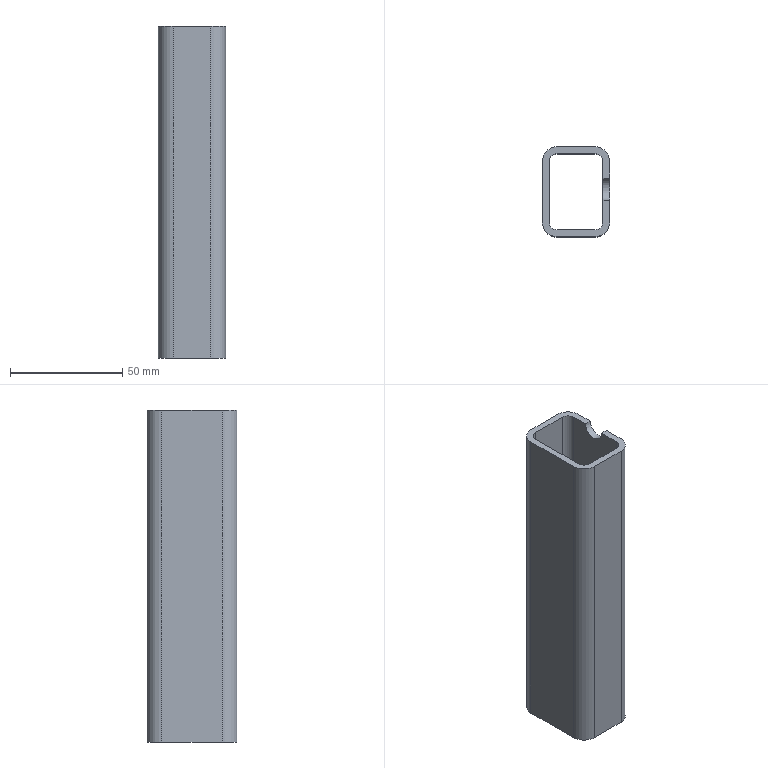Part | STEP file | DIN EN 10305-5 40 x 30 x 3 1785420022002 | 1 solid | 20 faces | box 30 x 40 x 147.63 mm | volume 52459 mm3 | cylinder 10 | plane 10 | commonest cylinder face diameters 7.2 x4 13.2 x4 10 x2
STEP:
#1=CARTESIAN_POINT('',(15.,-3.988,147.63));
#2=VERTEX_POINT('',#1);
#3=CARTESIAN_POINT('',(12.,-3.988,147.63));
#4=VERTEX_POINT('',#3);
#5=CARTESIAN_POINT('',(15.,-3.988,147.63));
#6=DIRECTION('',(-1.,0.,0.));
#7=VECTOR('',#6,10.);
#8=LINE('',#5,#7);
#9=EDGE_CURVE('',#2,#4,#8,.T.);
#10=ORIENTED_EDGE('',*,*,#9,.F.);
#11=CARTESIAN_POINT('',(15.,6.012,147.63));
#12=VERTEX_POINT('',#11);
#13=CARTESIAN_POINT('',(15.,1.012,147.63));
#14=DIRECTION('',(-1.,0.,0.));
#15=DIRECTION('',(0.,0.,-1.));
#16=AXIS2_PLACEMENT_3D('',#13,#14,#15);
#17=CIRCLE('',#16,5.);
#18=EDGE_CURVE('',#12,#2,#17,.T.);
#19=ORIENTED_EDGE('',*,*,#18,.F.);
#20=CARTESIAN_POINT('',(12.,6.012,147.63));
#21=VERTEX_POINT('',#20);
#22=CARTESIAN_POINT('',(15.,6.012,147.63));
#23=DIRECTION('',(1.,0.,0.));
#24=VECTOR('',#23,10.);
#25=LINE('',#22,#24);
#26=EDGE_CURVE('',#21,#12,#25,.T.);
#27=ORIENTED_EDGE('',*,*,#26,.F.);
#28=CARTESIAN_POINT('',(12.,1.012,147.63));
#29=DIRECTION('',(1.,0.,0.));
#30=DIRECTION('',(0.,0.,-1.));
#31=AXIS2_PLACEMENT_3D('',#28,#29,#30);
#32=CIRCLE('',#31,5.);
#33=EDGE_CURVE('',#4,#21,#32,.T.);
#34=ORIENTED_EDGE('',*,*,#33,.F.);
#35=EDGE_LOOP('',(#10,#19,#27,#34));
#36=FACE_OUTER_BOUND('',#35,.T.);
#37=CARTESIAN_POINT('',(15.,1.012,147.63));
#38=DIRECTION('',(-1.,0.,0.));
#39=DIRECTION('',(0.,0.,-1.));
#40=AXIS2_PLACEMENT_3D('',#37,#38,#39);
#41=CYLINDRICAL_SURFACE('',#40,5.);
#42=ADVANCED_FACE('',(#36),#41,.F.);
#43=CARTESIAN_POINT('',(15.,1.012,47.63));
#44=VERTEX_POINT('',#43);
#45=CARTESIAN_POINT('',(15.,1.012,42.63));
#46=DIRECTION('',(-1.,0.,0.));
#47=DIRECTION('',(0.,0.,-1.));
#48=AXIS2_PLACEMENT_3D('',#45,#46,#47);
#49=CIRCLE('',#48,5.);
#50=EDGE_CURVE('',#44,#44,#49,.T.);
#51=ORIENTED_EDGE('',*,*,#50,.F.);
#52=CARTESIAN_POINT('',(12.,1.012,47.63));
#53=VERTEX_POINT('',#52);
#54=CARTESIAN_POINT('',(15.,1.012,47.63));
#55=DIRECTION('',(-1.,0.,0.));
#56=VECTOR('',#55,5.);
#57=LINE('',#54,#56);
#58=EDGE_CURVE('',#44,#53,#57,.T.);
#59=ORIENTED_EDGE('',*,*,#58,.T.);
#60=CARTESIAN_POINT('',(12.,1.012,42.63));
#61=DIRECTION('',(1.,0.,0.));
#62=DIRECTION('',(0.,0.,-1.));
#63=AXIS2_PLACEMENT_3D('',#60,#61,#62);
#64=CIRCLE('',#63,5.);
#65=EDGE_CURVE('',#53,#53,#64,.T.);
#66=ORIENTED_EDGE('',*,*,#65,.F.);
#67=ORIENTED_EDGE('',*,*,#58,.F.);
#68=EDGE_LOOP('',(#51,#59,#66,#67));
#69=FACE_OUTER_BOUND('',#68,.T.);
#70=CARTESIAN_POINT('',(15.,1.012,42.63));
#71=DIRECTION('',(-1.,0.,0.));
#72=DIRECTION('',(0.,0.,-1.));
#73=AXIS2_PLACEMENT_3D('',#70,#71,#72);
#74=CYLINDRICAL_SURFACE('',#73,5.);
#75=ADVANCED_FACE('',(#69),#74,.F.);
#76=ORIENTED_EDGE('',*,*,#33,.T.);
#77=CARTESIAN_POINT('',(12.,13.4,147.63));
#78=VERTEX_POINT('',#77);
#79=CARTESIAN_POINT('',(12.,6.7,147.63));
#80=DIRECTION('',(0.,1.,0.));
#81=VECTOR('',#80,10.);
#82=LINE('',#79,#81);
#83=EDGE_CURVE('',#21,#78,#82,.T.);
#84=ORIENTED_EDGE('',*,*,#83,.T.);
#85=CARTESIAN_POINT('',(12.,13.4,0.));
#86=VERTEX_POINT('',#85);
#87=CARTESIAN_POINT('',(12.,13.4,0.));
#88=DIRECTION('',(0.,0.,1.));
#89=VECTOR('',#88,10.);
#90=LINE('',#87,#89);
#91=EDGE_CURVE('',#86,#78,#90,.T.);
#92=ORIENTED_EDGE('',*,*,#91,.F.);
#93=CARTESIAN_POINT('',(12.,-13.4,0.));
#94=VERTEX_POINT('',#93);
#95=CARTESIAN_POINT('',(12.,6.7,0.));
#96=DIRECTION('',(0.,1.,0.));
#97=VECTOR('',#96,10.);
#98=LINE('',#95,#97);
#99=EDGE_CURVE('',#94,#86,#98,.T.);
#100=ORIENTED_EDGE('',*,*,#99,.F.);
#101=CARTESIAN_POINT('',(12.,-13.4,147.63));
#102=VERTEX_POINT('',#101);
#103=CARTESIAN_POINT('',(12.,-13.4,0.));
#104=DIRECTION('',(0.,0.,1.));
#105=VECTOR('',#104,10.);
#106=LINE('',#103,#105);
#107=EDGE_CURVE('',#94,#102,#106,.T.);
#108=ORIENTED_EDGE('',*,*,#107,.T.);
#109=CARTESIAN_POINT('',(12.,6.7,147.63));
#110=DIRECTION('',(0.,1.,0.));
#111=VECTOR('',#110,10.);
#112=LINE('',#109,#111);
#113=EDGE_CURVE('',#102,#4,#112,.T.);
#114=ORIENTED_EDGE('',*,*,#113,.T.);
#115=EDGE_LOOP('',(#76,#84,#92,#100,#108,#114));
#116=FACE_OUTER_BOUND('',#115,.T.);
#117=ORIENTED_EDGE('',*,*,#65,.T.);
#118=EDGE_LOOP('',(#117));
#119=FACE_BOUND('',#118,.T.);
#120=CARTESIAN_POINT('',(12.,13.4,0.));
#121=DIRECTION('',(1.,0.,0.));
#122=DIRECTION('',(0.,0.,-1.));
#123=AXIS2_PLACEMENT_3D('',#120,#121,#122);
#124=PLANE('',#123);
#125=ADVANCED_FACE('',(#116,#119),#124,.F.);
#126=CARTESIAN_POINT('',(-8.4,-17.,147.63));
#127=VERTEX_POINT('',#126);
#128=CARTESIAN_POINT('',(8.4,-17.,147.63));
#129=VERTEX_POINT('',#128);
#130=CARTESIAN_POINT('',(4.2,-17.,147.63));
#131=DIRECTION('',(1.,0.,0.));
#132=VECTOR('',#131,10.);
#133=LINE('',#130,#132);
#134=EDGE_CURVE('',#127,#129,#133,.T.);
#135=ORIENTED_EDGE('',*,*,#134,.T.);
#136=CARTESIAN_POINT('',(8.4,-17.,0.));
#137=VERTEX_POINT('',#136);
#138=CARTESIAN_POINT('',(8.4,-17.,0.));
#139=DIRECTION('',(0.,0.,1.));
#140=VECTOR('',#139,10.);
#141=LINE('',#138,#140);
#142=EDGE_CURVE('',#137,#129,#141,.T.);
#143=ORIENTED_EDGE('',*,*,#142,.F.);
#144=CARTESIAN_POINT('',(-8.4,-17.,0.));
#145=VERTEX_POINT('',#144);
#146=CARTESIAN_POINT('',(4.2,-17.,0.));
#147=DIRECTION('',(1.,0.,0.));
#148=VECTOR('',#147,10.);
#149=LINE('',#146,#148);
#150=EDGE_CURVE('',#145,#137,#149,.T.);
#151=ORIENTED_EDGE('',*,*,#150,.F.);
#152=CARTESIAN_POINT('',(-8.4,-17.,0.));
#153=DIRECTION('',(0.,0.,1.));
#154=VECTOR('',#153,10.);
#155=LINE('',#152,#154);
#156=EDGE_CURVE('',#145,#127,#155,.T.);
#157=ORIENTED_EDGE('',*,*,#156,.T.);
#158=EDGE_LOOP('',(#135,#143,#151,#157));
#159=FACE_OUTER_BOUND('',#158,.T.);
#160=CARTESIAN_POINT('',(8.4,-17.,0.));
#161=DIRECTION('',(0.,-1.,0.));
#162=DIRECTION('',(0.,0.,-1.));
#163=AXIS2_PLACEMENT_3D('',#160,#161,#162);
#164=PLANE('',#163);
#165=ADVANCED_FACE('',(#159),#164,.F.);
#166=CARTESIAN_POINT('',(8.4,-13.4,147.63));
#167=DIRECTION('',(0.,0.,1.));
#168=DIRECTION('',(0.,1.,0.));
#169=AXIS2_PLACEMENT_3D('',#166,#167,#168);
#170=CIRCLE('',#169,3.6);
#171=EDGE_CURVE('',#129,#102,#170,.T.);
#172=ORIENTED_EDGE('',*,*,#171,.T.);
#173=ORIENTED_EDGE('',*,*,#107,.F.);
#174=CARTESIAN_POINT('',(8.4,-13.4,0.));
#175=DIRECTION('',(0.,0.,1.));
#176=DIRECTION('',(0.,1.,0.));
#177=AXIS2_PLACEMENT_3D('',#174,#175,#176);
#178=CIRCLE('',#177,3.6);
#179=EDGE_CURVE('',#137,#94,#178,.T.);
#180=ORIENTED_EDGE('',*,*,#179,.F.);
#181=ORIENTED_EDGE('',*,*,#142,.T.);
#182=EDGE_LOOP('',(#172,#173,#180,#181));
#183=FACE_OUTER_BOUND('',#182,.T.);
#184=CARTESIAN_POINT('',(8.4,-13.4,0.));
#185=DIRECTION('',(0.,0.,1.));
#186=DIRECTION('',(0.,1.,0.));
#187=AXIS2_PLACEMENT_3D('',#184,#185,#186);
#188=CYLINDRICAL_SURFACE('',#187,3.6);
#189=ADVANCED_FACE('',(#183),#188,.F.);
#190=CARTESIAN_POINT('',(8.4,17.,147.63));
#191=VERTEX_POINT('',#190);
#192=CARTESIAN_POINT('',(8.4,13.4,147.63));
#193=DIRECTION('',(0.,0.,1.));
#194=DIRECTION('',(-1.,0.,0.));
#195=AXIS2_PLACEMENT_3D('',#192,#193,#194);
#196=CIRCLE('',#195,3.6);
#197=EDGE_CURVE('',#78,#191,#196,.T.);
#198=ORIENTED_EDGE('',*,*,#197,.T.);
#199=CARTESIAN_POINT('',(8.4,17.,0.));
#200=VERTEX_POINT('',#199);
#201=CARTESIAN_POINT('',(8.4,17.,0.));
#202=DIRECTION('',(0.,0.,1.));
#203=VECTOR('',#202,10.);
#204=LINE('',#201,#203);
#205=EDGE_CURVE('',#200,#191,#204,.T.);
#206=ORIENTED_EDGE('',*,*,#205,.F.);
#207=CARTESIAN_POINT('',(8.4,13.4,0.));
#208=DIRECTION('',(0.,0.,1.));
#209=DIRECTION('',(-1.,0.,0.));
#210=AXIS2_PLACEMENT_3D('',#207,#208,#209);
#211=CIRCLE('',#210,3.6);
#212=EDGE_CURVE('',#86,#200,#211,.T.);
#213=ORIENTED_EDGE('',*,*,#212,.F.);
#214=ORIENTED_EDGE('',*,*,#91,.T.);
#215=EDGE_LOOP('',(#198,#206,#213,#214));
#216=FACE_OUTER_BOUND('',#215,.T.);
#217=CARTESIAN_POINT('',(8.4,13.4,0.));
#218=DIRECTION('',(0.,0.,1.));
#219=DIRECTION('',(-1.,0.,0.));
#220=AXIS2_PLACEMENT_3D('',#217,#218,#219);
#221=CYLINDRICAL_SURFACE('',#220,3.6);
#222=ADVANCED_FACE('',(#216),#221,.F.);
#223=ORIENTED_EDGE('',*,*,#18,.T.);
#224=CARTESIAN_POINT('',(15.,-13.4,147.63));
#225=VERTEX_POINT('',#224);
#226=CARTESIAN_POINT('',(15.,6.7,147.63));
#227=DIRECTION('',(0.,-1.,0.));
#228=VECTOR('',#227,10.);
#229=LINE('',#226,#228);
#230=EDGE_CURVE('',#2,#225,#229,.T.);
#231=ORIENTED_EDGE('',*,*,#230,.T.);
#232=CARTESIAN_POINT('',(15.,-13.4,0.));
#233=VERTEX_POINT('',#232);
#234=CARTESIAN_POINT('',(15.,-13.4,0.));
#235=DIRECTION('',(0.,0.,1.));
#236=VECTOR('',#235,10.);
#237=LINE('',#234,#236);
#238=EDGE_CURVE('',#233,#225,#237,.T.);
#239=ORIENTED_EDGE('',*,*,#238,.F.);
#240=CARTESIAN_POINT('',(15.,13.4,0.));
#241=VERTEX_POINT('',#240);
#242=CARTESIAN_POINT('',(15.,6.7,0.));
#243=DIRECTION('',(0.,-1.,0.));
#244=VECTOR('',#243,10.);
#245=LINE('',#242,#244);
#246=EDGE_CURVE('',#241,#233,#245,.T.);
#247=ORIENTED_EDGE('',*,*,#246,.F.);
#248=CARTESIAN_POINT('',(15.,13.4,147.63));
#249=VERTEX_POINT('',#248);
#250=CARTESIAN_POINT('',(15.,13.4,0.));
#251=DIRECTION('',(0.,0.,1.));
#252=VECTOR('',#251,10.);
#253=LINE('',#250,#252);
#254=EDGE_CURVE('',#241,#249,#253,.T.);
#255=ORIENTED_EDGE('',*,*,#254,.T.);
#256=CARTESIAN_POINT('',(15.,6.7,147.63));
#257=DIRECTION('',(0.,-1.,0.));
#258=VECTOR('',#257,10.);
#259=LINE('',#256,#258);
#260=EDGE_CURVE('',#249,#12,#259,.T.);
#261=ORIENTED_EDGE('',*,*,#260,.T.);
#262=EDGE_LOOP('',(#223,#231,#239,#247,#255,#261));
#263=FACE_OUTER_BOUND('',#262,.T.);
#264=ORIENTED_EDGE('',*,*,#50,.T.);
#265=EDGE_LOOP('',(#264));
#266=FACE_BOUND('',#265,.T.);
#267=CARTESIAN_POINT('',(15.,13.4,0.));
#268=DIRECTION('',(1.,0.,0.));
#269=DIRECTION('',(0.,0.,-1.));
#270=AXIS2_PLACEMENT_3D('',#267,#268,#269);
#271=PLANE('',#270);
#272=ADVANCED_FACE('',(#263,#266),#271,.T.);
#273=CARTESIAN_POINT('',(8.4,-20.,147.63));
#274=VERTEX_POINT('',#273);
#275=CARTESIAN_POINT('',(8.4,-13.4,147.63));
#276=DIRECTION('',(0.,0.,-1.));
#277=DIRECTION('',(0.,1.,0.));
#278=AXIS2_PLACEMENT_3D('',#275,#276,#277);
#279=CIRCLE('',#278,6.6);
#280=EDGE_CURVE('',#225,#274,#279,.T.);
#281=ORIENTED_EDGE('',*,*,#280,.T.);
#282=CARTESIAN_POINT('',(8.4,-20.,0.));
#283=VERTEX_POINT('',#282);
#284=CARTESIAN_POINT('',(8.4,-20.,0.));
#285=DIRECTION('',(0.,0.,1.));
#286=VECTOR('',#285,10.);
#287=LINE('',#284,#286);
#288=EDGE_CURVE('',#283,#274,#287,.T.);
#289=ORIENTED_EDGE('',*,*,#288,.F.);
#290=CARTESIAN_POINT('',(8.4,-13.4,0.));
#291=DIRECTION('',(0.,0.,-1.));
#292=DIRECTION('',(0.,1.,0.));
#293=AXIS2_PLACEMENT_3D('',#290,#291,#292);
#294=CIRCLE('',#293,6.6);
#295=EDGE_CURVE('',#233,#283,#294,.T.);
#296=ORIENTED_EDGE('',*,*,#295,.F.);
#297=ORIENTED_EDGE('',*,*,#238,.T.);
#298=EDGE_LOOP('',(#281,#289,#296,#297));
#299=FACE_OUTER_BOUND('',#298,.T.);
#300=CARTESIAN_POINT('',(8.4,-13.4,0.));
#301=DIRECTION('',(0.,0.,1.));
#302=DIRECTION('',(0.,1.,0.));
#303=AXIS2_PLACEMENT_3D('',#300,#301,#302);
#304=CYLINDRICAL_SURFACE('',#303,6.6);
#305=ADVANCED_FACE('',(#299),#304,.T.);
#306=CARTESIAN_POINT('',(-8.4,-20.,147.63));
#307=VERTEX_POINT('',#306);
#308=CARTESIAN_POINT('',(4.2,-20.,147.63));
#309=DIRECTION('',(-1.,0.,0.));
#310=VECTOR('',#309,10.);
#311=LINE('',#308,#310);
#312=EDGE_CURVE('',#274,#307,#311,.T.);
#313=ORIENTED_EDGE('',*,*,#312,.T.);
#314=CARTESIAN_POINT('',(-8.4,-20.,0.));
#315=VERTEX_POINT('',#314);
#316=CARTESIAN_POINT('',(-8.4,-20.,0.));
#317=DIRECTION('',(0.,0.,1.));
#318=VECTOR('',#317,10.);
#319=LINE('',#316,#318);
#320=EDGE_CURVE('',#315,#307,#319,.T.);
#321=ORIENTED_EDGE('',*,*,#320,.F.);
#322=CARTESIAN_POINT('',(4.2,-20.,0.));
#323=DIRECTION('',(-1.,0.,0.));
#324=VECTOR('',#323,10.);
#325=LINE('',#322,#324);
#326=EDGE_CURVE('',#283,#315,#325,.T.);
#327=ORIENTED_EDGE('',*,*,#326,.F.);
#328=ORIENTED_EDGE('',*,*,#288,.T.);
#329=EDGE_LOOP('',(#313,#321,#327,#328));
#330=FACE_OUTER_BOUND('',#329,.T.);
#331=CARTESIAN_POINT('',(8.4,-20.,0.));
#332=DIRECTION('',(0.,-1.,0.));
#333=DIRECTION('',(0.,0.,-1.));
#334=AXIS2_PLACEMENT_3D('',#331,#332,#333);
#335=PLANE('',#334);
#336=ADVANCED_FACE('',(#330),#335,.T.);
#337=CARTESIAN_POINT('',(-15.,-13.4,147.63));
#338=VERTEX_POINT('',#337);
#339=CARTESIAN_POINT('',(-8.4,-13.4,147.63));
#340=DIRECTION('',(0.,0.,-1.));
#341=DIRECTION('',(1.,0.,0.));
#342=AXIS2_PLACEMENT_3D('',#339,#340,#341);
#343=CIRCLE('',#342,6.6);
#344=EDGE_CURVE('',#307,#338,#343,.T.);
#345=ORIENTED_EDGE('',*,*,#344,.T.);
#346=CARTESIAN_POINT('',(-15.,-13.4,0.));
#347=VERTEX_POINT('',#346);
#348=CARTESIAN_POINT('',(-15.,-13.4,0.));
#349=DIRECTION('',(0.,0.,1.));
#350=VECTOR('',#349,10.);
#351=LINE('',#348,#350);
#352=EDGE_CURVE('',#347,#338,#351,.T.);
#353=ORIENTED_EDGE('',*,*,#352,.F.);
#354=CARTESIAN_POINT('',(-8.4,-13.4,0.));
#355=DIRECTION('',(0.,0.,-1.));
#356=DIRECTION('',(1.,0.,0.));
#357=AXIS2_PLACEMENT_3D('',#354,#355,#356);
#358=CIRCLE('',#357,6.6);
#359=EDGE_CURVE('',#315,#347,#358,.T.);
#360=ORIENTED_EDGE('',*,*,#359,.F.);
#361=ORIENTED_EDGE('',*,*,#320,.T.);
#362=EDGE_LOOP('',(#345,#353,#360,#361));
#363=FACE_OUTER_BOUND('',#362,.T.);
#364=CARTESIAN_POINT('',(-8.4,-13.4,0.));
#365=DIRECTION('',(0.,0.,1.));
#366=DIRECTION('',(1.,0.,0.));
#367=AXIS2_PLACEMENT_3D('',#364,#365,#366);
#368=CYLINDRICAL_SURFACE('',#367,6.6);
#369=ADVANCED_FACE('',(#363),#368,.T.);
#370=CARTESIAN_POINT('',(-8.4,17.,147.63));
#371=VERTEX_POINT('',#370);
#372=CARTESIAN_POINT('',(-4.2,17.,147.63));
#373=DIRECTION('',(-1.,0.,0.));
#374=VECTOR('',#373,10.);
#375=LINE('',#372,#374);
#376=EDGE_CURVE('',#191,#371,#375,.T.);
#377=ORIENTED_EDGE('',*,*,#376,.T.);
#378=CARTESIAN_POINT('',(-8.4,17.,0.));
#379=VERTEX_POINT('',#378);
#380=CARTESIAN_POINT('',(-8.4,17.,0.));
#381=DIRECTION('',(0.,0.,1.));
#382=VECTOR('',#381,10.);
#383=LINE('',#380,#382);
#384=EDGE_CURVE('',#379,#371,#383,.T.);
#385=ORIENTED_EDGE('',*,*,#384,.F.);
#386=CARTESIAN_POINT('',(-4.2,17.,0.));
#387=DIRECTION('',(-1.,0.,0.));
#388=VECTOR('',#387,10.);
#389=LINE('',#386,#388);
#390=EDGE_CURVE('',#200,#379,#389,.T.);
#391=ORIENTED_EDGE('',*,*,#390,.F.);
#392=ORIENTED_EDGE('',*,*,#205,.T.);
#393=EDGE_LOOP('',(#377,#385,#391,#392));
#394=FACE_OUTER_BOUND('',#393,.T.);
#395=CARTESIAN_POINT('',(-8.4,17.,0.));
#396=DIRECTION('',(0.,1.,0.));
#397=DIRECTION('',(0.,0.,1.));
#398=AXIS2_PLACEMENT_3D('',#395,#396,#397);
#399=PLANE('',#398);
#400=ADVANCED_FACE('',(#394),#399,.F.);
#401=CARTESIAN_POINT('',(-12.,-13.4,147.63));
#402=VERTEX_POINT('',#401);
#403=CARTESIAN_POINT('',(-8.4,-13.4,147.63));
#404=DIRECTION('',(0.,0.,1.));
#405=DIRECTION('',(1.,0.,0.));
#406=AXIS2_PLACEMENT_3D('',#403,#404,#405);
#407=CIRCLE('',#406,3.6);
#408=EDGE_CURVE('',#402,#127,#407,.T.);
#409=ORIENTED_EDGE('',*,*,#408,.T.);
#410=ORIENTED_EDGE('',*,*,#156,.F.);
#411=CARTESIAN_POINT('',(-12.,-13.4,0.));
#412=VERTEX_POINT('',#411);
#413=CARTESIAN_POINT('',(-8.4,-13.4,0.));
#414=DIRECTION('',(0.,0.,1.));
#415=DIRECTION('',(1.,0.,0.));
#416=AXIS2_PLACEMENT_3D('',#413,#414,#415);
#417=CIRCLE('',#416,3.6);
#418=EDGE_CURVE('',#412,#145,#417,.T.);
#419=ORIENTED_EDGE('',*,*,#418,.F.);
#420=CARTESIAN_POINT('',(-12.,-13.4,0.));
#421=DIRECTION('',(0.,0.,1.));
#422=VECTOR('',#421,10.);
#423=LINE('',#420,#422);
#424=EDGE_CURVE('',#412,#402,#423,.T.);
#425=ORIENTED_EDGE('',*,*,#424,.T.);
#426=EDGE_LOOP('',(#409,#410,#419,#425));
#427=FACE_OUTER_BOUND('',#426,.T.);
#428=CARTESIAN_POINT('',(-8.4,-13.4,0.));
#429=DIRECTION('',(0.,0.,1.));
#430=DIRECTION('',(1.,0.,0.));
#431=AXIS2_PLACEMENT_3D('',#428,#429,#430);
#432=CYLINDRICAL_SURFACE('',#431,3.6);
#433=ADVANCED_FACE('',(#427),#432,.F.);
#434=CARTESIAN_POINT('',(-12.,13.4,147.63));
#435=VERTEX_POINT('',#434);
#436=CARTESIAN_POINT('',(-12.,-6.7,147.63));
#437=DIRECTION('',(0.,-1.,0.));
#438=VECTOR('',#437,10.);
#439=LINE('',#436,#438);
#440=EDGE_CURVE('',#435,#402,#439,.T.);
#441=ORIENTED_EDGE('',*,*,#440,.T.);
#442=ORIENTED_EDGE('',*,*,#424,.F.);
#443=CARTESIAN_POINT('',(-12.,13.4,0.));
#444=VERTEX_POINT('',#443);
#445=CARTESIAN_POINT('',(-12.,-6.7,0.));
#446=DIRECTION('',(0.,-1.,0.));
#447=VECTOR('',#446,10.);
#448=LINE('',#445,#447);
#449=EDGE_CURVE('',#444,#412,#448,.T.);
#450=ORIENTED_EDGE('',*,*,#449,.F.);
#451=CARTESIAN_POINT('',(-12.,13.4,0.));
#452=DIRECTION('',(0.,0.,1.));
#453=VECTOR('',#452,10.);
#454=LINE('',#451,#453);
#455=EDGE_CURVE('',#444,#435,#454,.T.);
#456=ORIENTED_EDGE('',*,*,#455,.T.);
#457=EDGE_LOOP('',(#441,#442,#450,#456));
#458=FACE_OUTER_BOUND('',#457,.T.);
#459=CARTESIAN_POINT('',(-12.,-13.4,0.));
#460=DIRECTION('',(-1.,0.,0.));
#461=DIRECTION('',(0.,0.,1.));
#462=AXIS2_PLACEMENT_3D('',#459,#460,#461);
#463=PLANE('',#462);
#464=ADVANCED_FACE('',(#458),#463,.F.);
#465=CARTESIAN_POINT('',(-8.4,13.4,147.63));
#466=DIRECTION('',(0.,0.,1.));
#467=DIRECTION('',(0.,-1.,0.));
#468=AXIS2_PLACEMENT_3D('',#465,#466,#467);
#469=CIRCLE('',#468,3.6);
#470=EDGE_CURVE('',#371,#435,#469,.T.);
#471=ORIENTED_EDGE('',*,*,#470,.T.);
#472=ORIENTED_EDGE('',*,*,#455,.F.);
#473=CARTESIAN_POINT('',(-8.4,13.4,0.));
#474=DIRECTION('',(0.,0.,1.));
#475=DIRECTION('',(0.,-1.,0.));
#476=AXIS2_PLACEMENT_3D('',#473,#474,#475);
#477=CIRCLE('',#476,3.6);
#478=EDGE_CURVE('',#379,#444,#477,.T.);
#479=ORIENTED_EDGE('',*,*,#478,.F.);
#480=ORIENTED_EDGE('',*,*,#384,.T.);
#481=EDGE_LOOP('',(#471,#472,#479,#480));
#482=FACE_OUTER_BOUND('',#481,.T.);
#483=CARTESIAN_POINT('',(-8.4,13.4,0.));
#484=DIRECTION('',(0.,0.,1.));
#485=DIRECTION('',(0.,-1.,0.));
#486=AXIS2_PLACEMENT_3D('',#483,#484,#485);
#487=CYLINDRICAL_SURFACE('',#486,3.6);
#488=ADVANCED_FACE('',(#482),#487,.F.);
#489=CARTESIAN_POINT('',(-15.,13.4,147.63));
#490=VERTEX_POINT('',#489);
#491=CARTESIAN_POINT('',(-15.,-6.7,147.63));
#492=DIRECTION('',(0.,1.,0.));
#493=VECTOR('',#492,10.);
#494=LINE('',#491,#493);
#495=EDGE_CURVE('',#338,#490,#494,.T.);
#496=ORIENTED_EDGE('',*,*,#495,.T.);
#497=CARTESIAN_POINT('',(-15.,13.4,0.));
#498=VERTEX_POINT('',#497);
#499=CARTESIAN_POINT('',(-15.,13.4,0.));
#500=DIRECTION('',(0.,0.,1.));
#501=VECTOR('',#500,10.);
#502=LINE('',#499,#501);
#503=EDGE_CURVE('',#498,#490,#502,.T.);
#504=ORIENTED_EDGE('',*,*,#503,.F.);
#505=CARTESIAN_POINT('',(-15.,-6.7,0.));
#506=DIRECTION('',(0.,1.,0.));
#507=VECTOR('',#506,10.);
#508=LINE('',#505,#507);
#509=EDGE_CURVE('',#347,#498,#508,.T.);
#510=ORIENTED_EDGE('',*,*,#509,.F.);
#511=ORIENTED_EDGE('',*,*,#352,.T.);
#512=EDGE_LOOP('',(#496,#504,#510,#511));
#513=FACE_OUTER_BOUND('',#512,.T.);
#514=CARTESIAN_POINT('',(-15.,-13.4,0.));
#515=DIRECTION('',(-1.,0.,0.));
#516=DIRECTION('',(0.,0.,1.));
#517=AXIS2_PLACEMENT_3D('',#514,#515,#516);
#518=PLANE('',#517);
#519=ADVANCED_FACE('',(#513),#518,.T.);
#520=CARTESIAN_POINT('',(-8.4,20.,147.63));
#521=VERTEX_POINT('',#520);
#522=CARTESIAN_POINT('',(-8.4,13.4,147.63));
#523=DIRECTION('',(0.,0.,-1.));
#524=DIRECTION('',(0.,-1.,0.));
#525=AXIS2_PLACEMENT_3D('',#522,#523,#524);
#526=CIRCLE('',#525,6.6);
#527=EDGE_CURVE('',#490,#521,#526,.T.);
#528=ORIENTED_EDGE('',*,*,#527,.T.);
#529=CARTESIAN_POINT('',(-8.4,20.,0.));
#530=VERTEX_POINT('',#529);
#531=CARTESIAN_POINT('',(-8.4,20.,0.));
#532=DIRECTION('',(0.,0.,1.));
#533=VECTOR('',#532,10.);
#534=LINE('',#531,#533);
#535=EDGE_CURVE('',#530,#521,#534,.T.);
#536=ORIENTED_EDGE('',*,*,#535,.F.);
#537=CARTESIAN_POINT('',(-8.4,13.4,0.));
#538=DIRECTION('',(0.,0.,-1.));
#539=DIRECTION('',(0.,-1.,0.));
#540=AXIS2_PLACEMENT_3D('',#537,#538,#539);
#541=CIRCLE('',#540,6.6);
#542=EDGE_CURVE('',#498,#530,#541,.T.);
#543=ORIENTED_EDGE('',*,*,#542,.F.);
#544=ORIENTED_EDGE('',*,*,#503,.T.);
#545=EDGE_LOOP('',(#528,#536,#543,#544));
#546=FACE_OUTER_BOUND('',#545,.T.);
#547=CARTESIAN_POINT('',(-8.4,13.4,0.));
#548=DIRECTION('',(0.,0.,1.));
#549=DIRECTION('',(0.,-1.,0.));
#550=AXIS2_PLACEMENT_3D('',#547,#548,#549);
#551=CYLINDRICAL_SURFACE('',#550,6.6);
#552=ADVANCED_FACE('',(#546),#551,.T.);
#553=CARTESIAN_POINT('',(8.4,20.,147.63));
#554=VERTEX_POINT('',#553);
#555=CARTESIAN_POINT('',(-4.2,20.,147.63));
#556=DIRECTION('',(1.,0.,0.));
#557=VECTOR('',#556,10.);
#558=LINE('',#555,#557);
#559=EDGE_CURVE('',#521,#554,#558,.T.);
#560=ORIENTED_EDGE('',*,*,#559,.T.);
#561=CARTESIAN_POINT('',(8.4,20.,0.));
#562=VERTEX_POINT('',#561);
#563=CARTESIAN_POINT('',(8.4,20.,0.));
#564=DIRECTION('',(0.,0.,1.));
#565=VECTOR('',#564,10.);
#566=LINE('',#563,#565);
#567=EDGE_CURVE('',#562,#554,#566,.T.);
#568=ORIENTED_EDGE('',*,*,#567,.F.);
#569=CARTESIAN_POINT('',(-4.2,20.,0.));
#570=DIRECTION('',(1.,0.,0.));
#571=VECTOR('',#570,10.);
#572=LINE('',#569,#571);
#573=EDGE_CURVE('',#530,#562,#572,.T.);
#574=ORIENTED_EDGE('',*,*,#573,.F.);
#575=ORIENTED_EDGE('',*,*,#535,.T.);
#576=EDGE_LOOP('',(#560,#568,#574,#575));
#577=FACE_OUTER_BOUND('',#576,.T.);
#578=CARTESIAN_POINT('',(-8.4,20.,0.));
#579=DIRECTION('',(0.,1.,0.));
#580=DIRECTION('',(0.,0.,1.));
#581=AXIS2_PLACEMENT_3D('',#578,#579,#580);
#582=PLANE('',#581);
#583=ADVANCED_FACE('',(#577),#582,.T.);
#584=CARTESIAN_POINT('',(8.4,13.4,147.63));
#585=DIRECTION('',(0.,0.,-1.));
#586=DIRECTION('',(-1.,0.,0.));
#587=AXIS2_PLACEMENT_3D('',#584,#585,#586);
#588=CIRCLE('',#587,6.6);
#589=EDGE_CURVE('',#554,#249,#588,.T.);
#590=ORIENTED_EDGE('',*,*,#589,.T.);
#591=ORIENTED_EDGE('',*,*,#254,.F.);
#592=CARTESIAN_POINT('',(8.4,13.4,0.));
#593=DIRECTION('',(0.,0.,-1.));
#594=DIRECTION('',(-1.,0.,0.));
#595=AXIS2_PLACEMENT_3D('',#592,#593,#594);
#596=CIRCLE('',#595,6.6);
#597=EDGE_CURVE('',#562,#241,#596,.T.);
#598=ORIENTED_EDGE('',*,*,#597,.F.);
#599=ORIENTED_EDGE('',*,*,#567,.T.);
#600=EDGE_LOOP('',(#590,#591,#598,#599));
#601=FACE_OUTER_BOUND('',#600,.T.);
#602=CARTESIAN_POINT('',(8.4,13.4,0.));
#603=DIRECTION('',(0.,0.,1.));
#604=DIRECTION('',(-1.,0.,0.));
#605=AXIS2_PLACEMENT_3D('',#602,#603,#604);
#606=CYLINDRICAL_SURFACE('',#605,6.6);
#607=ADVANCED_FACE('',(#601),#606,.T.);
#608=ORIENTED_EDGE('',*,*,#509,.T.);
#609=ORIENTED_EDGE('',*,*,#542,.T.);
#610=ORIENTED_EDGE('',*,*,#573,.T.);
#611=ORIENTED_EDGE('',*,*,#597,.T.);
#612=ORIENTED_EDGE('',*,*,#246,.T.);
#613=ORIENTED_EDGE('',*,*,#295,.T.);
#614=ORIENTED_EDGE('',*,*,#326,.T.);
#615=ORIENTED_EDGE('',*,*,#359,.T.);
#616=EDGE_LOOP('',(#608,#609,#610,#611,#612,#613,#614,#615));
#617=FACE_OUTER_BOUND('',#616,.T.);
#618=ORIENTED_EDGE('',*,*,#390,.T.);
#619=ORIENTED_EDGE('',*,*,#478,.T.);
#620=ORIENTED_EDGE('',*,*,#449,.T.);
#621=ORIENTED_EDGE('',*,*,#418,.T.);
#622=ORIENTED_EDGE('',*,*,#150,.T.);
#623=ORIENTED_EDGE('',*,*,#179,.T.);
#624=ORIENTED_EDGE('',*,*,#99,.T.);
#625=ORIENTED_EDGE('',*,*,#212,.T.);
#626=EDGE_LOOP('',(#618,#619,#620,#621,#622,#623,#624,#625));
#627=FACE_BOUND('',#626,.T.);
#628=CARTESIAN_POINT('',(0.,0.,0.));
#629=DIRECTION('',(0.,0.,1.));
#630=DIRECTION('',(1.,0.,0.));
#631=AXIS2_PLACEMENT_3D('',#628,#629,#630);
#632=PLANE('',#631);
#633=ADVANCED_FACE('',(#617,#627),#632,.F.);
#634=ORIENTED_EDGE('',*,*,#9,.T.);
#635=ORIENTED_EDGE('',*,*,#113,.F.);
#636=ORIENTED_EDGE('',*,*,#171,.F.);
#637=ORIENTED_EDGE('',*,*,#134,.F.);
#638=ORIENTED_EDGE('',*,*,#408,.F.);
#639=ORIENTED_EDGE('',*,*,#440,.F.);
#640=ORIENTED_EDGE('',*,*,#470,.F.);
#641=ORIENTED_EDGE('',*,*,#376,.F.);
#642=ORIENTED_EDGE('',*,*,#197,.F.);
#643=ORIENTED_EDGE('',*,*,#83,.F.);
#644=ORIENTED_EDGE('',*,*,#26,.T.);
#645=ORIENTED_EDGE('',*,*,#260,.F.);
#646=ORIENTED_EDGE('',*,*,#589,.F.);
#647=ORIENTED_EDGE('',*,*,#559,.F.);
#648=ORIENTED_EDGE('',*,*,#527,.F.);
#649=ORIENTED_EDGE('',*,*,#495,.F.);
#650=ORIENTED_EDGE('',*,*,#344,.F.);
#651=ORIENTED_EDGE('',*,*,#312,.F.);
#652=ORIENTED_EDGE('',*,*,#280,.F.);
#653=ORIENTED_EDGE('',*,*,#230,.F.);
#654=EDGE_LOOP('',(#634,#635,#636,#637,#638,#639,#640,#641,#642,#643,#644,#645,#646,#647,#648,#649,#650,#651,#652,#653));
#655=FACE_OUTER_BOUND('',#654,.T.);
#656=CARTESIAN_POINT('',(0.,0.,147.63));
#657=DIRECTION('',(0.,0.,1.));
#658=DIRECTION('',(1.,0.,0.));
#659=AXIS2_PLACEMENT_3D('',#656,#657,#658);
#660=PLANE('',#659);
#661=ADVANCED_FACE('',(#655),#660,.T.);
#662=CLOSED_SHELL('',(#42,#75,#125,#165,#189,#222,#272,#305,#336,#369,#400,#433,#464,#488,#519,#552,#583,#607,#633,#661));
#663=MANIFOLD_SOLID_BREP('',#662);
#664=(LENGTH_UNIT()NAMED_UNIT(*)SI_UNIT(.MILLI.,.METRE.));
#665=UNCERTAINTY_MEASURE_WITH_UNIT(LENGTH_MEASURE(0.01),#664,'','');
#666=(NAMED_UNIT(*)PLANE_ANGLE_UNIT()SI_UNIT($,.RADIAN.));
#667=(NAMED_UNIT(*)SI_UNIT($,.STERADIAN.)SOLID_ANGLE_UNIT());
#668=(GEOMETRIC_REPRESENTATION_CONTEXT(3)GLOBAL_UNCERTAINTY_ASSIGNED_CONTEXT((#665))GLOBAL_UNIT_ASSIGNED_CONTEXT((#664,#666,#667))REPRESENTATION_CONTEXT('',''));
#669=ADVANCED_BREP_SHAPE_REPRESENTATION('',(#663),#668);